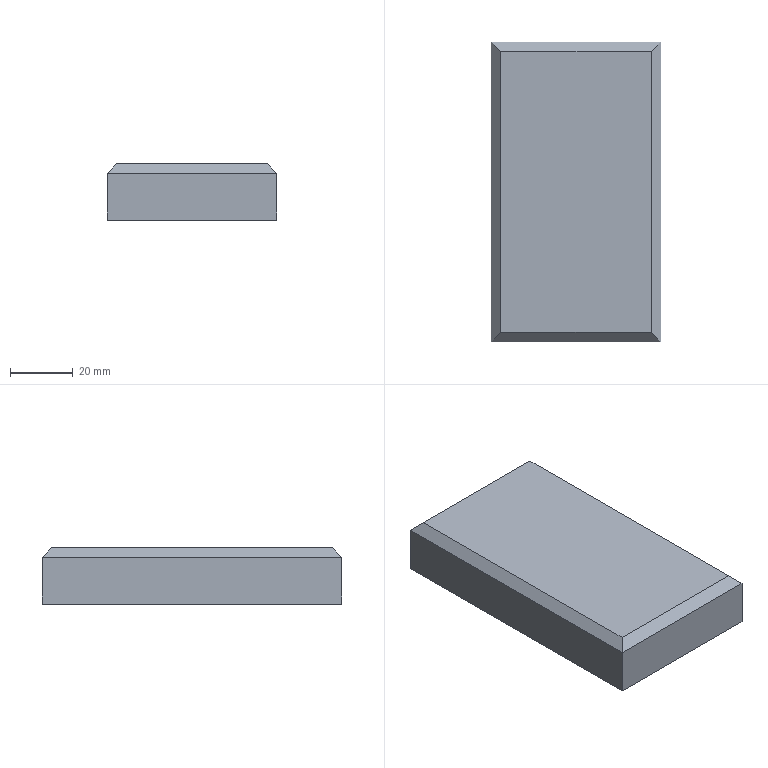Part | NX | 1 solid | 10 faces | box 54.267 x 95.886 x 18 mm | volume 92346 mm3 | plane 10
STEP:
#1=CARTESIAN_POINT('',(-11.284,-691.843,2485.086));
#2=VERTEX_POINT('',#1);
#3=CARTESIAN_POINT('',(-11.284,-691.843,2500.086));
#4=VERTEX_POINT('',#3);
#5=CARTESIAN_POINT('',(-11.284,-691.843,2485.086));
#6=DIRECTION('',(0.,0.,1.));
#7=VECTOR('',#6,1.);
#8=LINE('',#5,#7);
#9=EDGE_CURVE('',#2,#4,#8,.T.);
#10=ORIENTED_EDGE('',*,*,#9,.T.);
#11=CARTESIAN_POINT('',(-11.284,-595.957,2500.086));
#12=VERTEX_POINT('',#11);
#13=CARTESIAN_POINT('',(-11.284,-595.957,2500.086));
#14=DIRECTION('',(0.,1.,0.));
#15=VECTOR('',#14,1.);
#16=LINE('',#13,#15);
#17=EDGE_CURVE('',#4,#12,#16,.T.);
#18=ORIENTED_EDGE('',*,*,#17,.T.);
#19=CARTESIAN_POINT('',(-11.284,-595.957,2485.086));
#20=VERTEX_POINT('',#19);
#21=CARTESIAN_POINT('',(-11.284,-595.957,2485.086));
#22=DIRECTION('',(0.,0.,1.));
#23=VECTOR('',#22,1.);
#24=LINE('',#21,#23);
#25=EDGE_CURVE('',#20,#12,#24,.T.);
#26=ORIENTED_EDGE('',*,*,#25,.F.);
#27=CARTESIAN_POINT('',(-11.284,-595.957,2485.086));
#28=DIRECTION('',(0.,-1.,0.));
#29=VECTOR('',#28,1.);
#30=LINE('',#27,#29);
#31=EDGE_CURVE('',#20,#2,#30,.T.);
#32=ORIENTED_EDGE('',*,*,#31,.T.);
#33=EDGE_LOOP('',(#10,#18,#26,#32));
#34=FACE_OUTER_BOUND('',#33,.T.);
#35=CARTESIAN_POINT('',(-11.284,-595.957,2485.086));
#36=DIRECTION('',(-1.,0.,0.));
#37=DIRECTION('',(0.,-1.,0.));
#38=AXIS2_PLACEMENT_3D('',#35,#36,#37);
#39=PLANE('',#38);
#40=ADVANCED_FACE('',(#34),#39,.T.);
#41=ORIENTED_EDGE('',*,*,#25,.T.);
#42=CARTESIAN_POINT('',(42.983,-595.957,2500.086));
#43=VERTEX_POINT('',#42);
#44=CARTESIAN_POINT('',(-11.284,-595.957,2500.086));
#45=DIRECTION('',(1.,0.,0.));
#46=VECTOR('',#45,1.);
#47=LINE('',#44,#46);
#48=EDGE_CURVE('',#12,#43,#47,.T.);
#49=ORIENTED_EDGE('',*,*,#48,.T.);
#50=CARTESIAN_POINT('',(42.983,-595.957,2485.086));
#51=VERTEX_POINT('',#50);
#52=CARTESIAN_POINT('',(42.983,-595.957,2485.086));
#53=DIRECTION('',(0.,0.,1.));
#54=VECTOR('',#53,1.);
#55=LINE('',#52,#54);
#56=EDGE_CURVE('',#51,#43,#55,.T.);
#57=ORIENTED_EDGE('',*,*,#56,.F.);
#58=CARTESIAN_POINT('',(-11.284,-595.957,2485.086));
#59=DIRECTION('',(-1.,0.,0.));
#60=VECTOR('',#59,1.);
#61=LINE('',#58,#60);
#62=EDGE_CURVE('',#51,#20,#61,.T.);
#63=ORIENTED_EDGE('',*,*,#62,.T.);
#64=EDGE_LOOP('',(#41,#49,#57,#63));
#65=FACE_OUTER_BOUND('',#64,.T.);
#66=CARTESIAN_POINT('',(-11.284,-595.957,2485.086));
#67=DIRECTION('',(0.,1.,0.));
#68=DIRECTION('',(0.,0.,1.));
#69=AXIS2_PLACEMENT_3D('',#66,#67,#68);
#70=PLANE('',#69);
#71=ADVANCED_FACE('',(#65),#70,.T.);
#72=ORIENTED_EDGE('',*,*,#56,.T.);
#73=CARTESIAN_POINT('',(42.983,-691.843,2500.086));
#74=VERTEX_POINT('',#73);
#75=CARTESIAN_POINT('',(42.983,-595.957,2500.086));
#76=DIRECTION('',(0.,-1.,0.));
#77=VECTOR('',#76,1.);
#78=LINE('',#75,#77);
#79=EDGE_CURVE('',#43,#74,#78,.T.);
#80=ORIENTED_EDGE('',*,*,#79,.T.);
#81=CARTESIAN_POINT('',(42.983,-691.843,2485.086));
#82=VERTEX_POINT('',#81);
#83=CARTESIAN_POINT('',(42.983,-691.843,2485.086));
#84=DIRECTION('',(0.,0.,1.));
#85=VECTOR('',#84,1.);
#86=LINE('',#83,#85);
#87=EDGE_CURVE('',#82,#74,#86,.T.);
#88=ORIENTED_EDGE('',*,*,#87,.F.);
#89=CARTESIAN_POINT('',(42.983,-595.957,2485.086));
#90=DIRECTION('',(0.,1.,0.));
#91=VECTOR('',#90,1.);
#92=LINE('',#89,#91);
#93=EDGE_CURVE('',#82,#51,#92,.T.);
#94=ORIENTED_EDGE('',*,*,#93,.T.);
#95=EDGE_LOOP('',(#72,#80,#88,#94));
#96=FACE_OUTER_BOUND('',#95,.T.);
#97=CARTESIAN_POINT('',(42.983,-595.957,2485.086));
#98=DIRECTION('',(1.,0.,0.));
#99=DIRECTION('',(0.,0.,-1.));
#100=AXIS2_PLACEMENT_3D('',#97,#98,#99);
#101=PLANE('',#100);
#102=ADVANCED_FACE('',(#96),#101,.T.);
#103=ORIENTED_EDGE('',*,*,#87,.T.);
#104=CARTESIAN_POINT('',(-11.284,-691.843,2500.086));
#105=DIRECTION('',(-1.,0.,0.));
#106=VECTOR('',#105,1.);
#107=LINE('',#104,#106);
#108=EDGE_CURVE('',#74,#4,#107,.T.);
#109=ORIENTED_EDGE('',*,*,#108,.T.);
#110=ORIENTED_EDGE('',*,*,#9,.F.);
#111=CARTESIAN_POINT('',(-11.284,-691.843,2485.086));
#112=DIRECTION('',(1.,0.,0.));
#113=VECTOR('',#112,1.);
#114=LINE('',#111,#113);
#115=EDGE_CURVE('',#2,#82,#114,.T.);
#116=ORIENTED_EDGE('',*,*,#115,.T.);
#117=EDGE_LOOP('',(#103,#109,#110,#116));
#118=FACE_OUTER_BOUND('',#117,.T.);
#119=CARTESIAN_POINT('',(-11.284,-691.843,2485.086));
#120=DIRECTION('',(0.,-1.,0.));
#121=DIRECTION('',(0.,0.,-1.));
#122=AXIS2_PLACEMENT_3D('',#119,#120,#121);
#123=PLANE('',#122);
#124=ADVANCED_FACE('',(#118),#123,.T.);
#125=ORIENTED_EDGE('',*,*,#31,.F.);
#126=ORIENTED_EDGE('',*,*,#62,.F.);
#127=ORIENTED_EDGE('',*,*,#93,.F.);
#128=ORIENTED_EDGE('',*,*,#115,.F.);
#129=EDGE_LOOP('',(#125,#126,#127,#128));
#130=FACE_OUTER_BOUND('',#129,.T.);
#131=CARTESIAN_POINT('',(-11.284,-691.843,2485.086));
#132=DIRECTION('',(0.,0.,1.));
#133=DIRECTION('',(1.,0.,0.));
#134=AXIS2_PLACEMENT_3D('',#131,#132,#133);
#135=PLANE('',#134);
#136=ADVANCED_FACE('',(#130),#135,.F.);
#137=CARTESIAN_POINT('',(39.983,-688.843,2503.086));
#138=VERTEX_POINT('',#137);
#139=CARTESIAN_POINT('',(39.983,-598.957,2503.086));
#140=VERTEX_POINT('',#139);
#141=CARTESIAN_POINT('',(39.983,-691.843,2503.086));
#142=DIRECTION('',(0.,1.,0.));
#143=VECTOR('',#142,1.);
#144=LINE('',#141,#143);
#145=EDGE_CURVE('',#138,#140,#144,.T.);
#146=ORIENTED_EDGE('',*,*,#145,.T.);
#147=CARTESIAN_POINT('',(-8.284,-598.957,2503.086));
#148=VERTEX_POINT('',#147);
#149=CARTESIAN_POINT('',(-11.284,-598.957,2503.086));
#150=DIRECTION('',(-1.,0.,0.));
#151=VECTOR('',#150,1.);
#152=LINE('',#149,#151);
#153=EDGE_CURVE('',#140,#148,#152,.T.);
#154=ORIENTED_EDGE('',*,*,#153,.T.);
#155=CARTESIAN_POINT('',(-8.284,-688.843,2503.086));
#156=VERTEX_POINT('',#155);
#157=CARTESIAN_POINT('',(-8.284,-691.843,2503.086));
#158=DIRECTION('',(0.,-1.,0.));
#159=VECTOR('',#158,1.);
#160=LINE('',#157,#159);
#161=EDGE_CURVE('',#148,#156,#160,.T.);
#162=ORIENTED_EDGE('',*,*,#161,.T.);
#163=CARTESIAN_POINT('',(-11.284,-688.843,2503.086));
#164=DIRECTION('',(1.,0.,0.));
#165=VECTOR('',#164,1.);
#166=LINE('',#163,#165);
#167=EDGE_CURVE('',#156,#138,#166,.T.);
#168=ORIENTED_EDGE('',*,*,#167,.T.);
#169=EDGE_LOOP('',(#146,#154,#162,#168));
#170=FACE_OUTER_BOUND('',#169,.T.);
#171=CARTESIAN_POINT('',(-11.284,-691.843,2503.086));
#172=DIRECTION('',(0.,0.,1.));
#173=DIRECTION('',(1.,0.,0.));
#174=AXIS2_PLACEMENT_3D('',#171,#172,#173);
#175=PLANE('',#174);
#176=ADVANCED_FACE('',(#170),#175,.T.);
#177=CARTESIAN_POINT('',(-9.284,-689.843,2502.086));
#178=DIRECTION('',(0.5774,0.5774,0.5774));
#179=VECTOR('',#178,1.);
#180=LINE('',#177,#179);
#181=EDGE_CURVE('',#4,#156,#180,.T.);
#182=ORIENTED_EDGE('',*,*,#181,.F.);
#183=ORIENTED_EDGE('',*,*,#108,.F.);
#184=CARTESIAN_POINT('',(22.894,-671.754,2520.175));
#185=DIRECTION('',(0.5774,-0.5774,-0.5774));
#186=VECTOR('',#185,1.);
#187=LINE('',#184,#186);
#188=EDGE_CURVE('',#138,#74,#187,.T.);
#189=ORIENTED_EDGE('',*,*,#188,.F.);
#190=ORIENTED_EDGE('',*,*,#167,.F.);
#191=EDGE_LOOP('',(#182,#183,#189,#190));
#192=FACE_OUTER_BOUND('',#191,.T.);
#193=CARTESIAN_POINT('',(-11.284,-688.843,2503.086));
#194=DIRECTION('',(0.,0.7071,-0.7071));
#195=DIRECTION('',(0.,0.7071,0.7071));
#196=AXIS2_PLACEMENT_3D('',#193,#194,#195);
#197=PLANE('',#196);
#198=ADVANCED_FACE('',(#192),#197,.F.);
#199=ORIENTED_EDGE('',*,*,#188,.T.);
#200=ORIENTED_EDGE('',*,*,#79,.F.);
#201=CARTESIAN_POINT('',(9.021,-629.919,2534.048));
#202=DIRECTION('',(0.5774,0.5774,-0.5774));
#203=VECTOR('',#202,1.);
#204=LINE('',#201,#203);
#205=EDGE_CURVE('',#140,#43,#204,.T.);
#206=ORIENTED_EDGE('',*,*,#205,.F.);
#207=ORIENTED_EDGE('',*,*,#145,.F.);
#208=EDGE_LOOP('',(#199,#200,#206,#207));
#209=FACE_OUTER_BOUND('',#208,.T.);
#210=CARTESIAN_POINT('',(39.983,-691.843,2503.086));
#211=DIRECTION('',(-0.7071,0.,-0.7071));
#212=DIRECTION('',(-0.7071,0.,0.7071));
#213=AXIS2_PLACEMENT_3D('',#210,#211,#212);
#214=PLANE('',#213);
#215=ADVANCED_FACE('',(#209),#214,.F.);
#216=ORIENTED_EDGE('',*,*,#181,.T.);
#217=ORIENTED_EDGE('',*,*,#161,.F.);
#218=CARTESIAN_POINT('',(22.678,-629.919,2534.048));
#219=DIRECTION('',(0.5774,-0.5774,0.5774));
#220=VECTOR('',#219,1.);
#221=LINE('',#218,#220);
#222=EDGE_CURVE('',#12,#148,#221,.T.);
#223=ORIENTED_EDGE('',*,*,#222,.F.);
#224=ORIENTED_EDGE('',*,*,#17,.F.);
#225=EDGE_LOOP('',(#216,#217,#223,#224));
#226=FACE_OUTER_BOUND('',#225,.T.);
#227=CARTESIAN_POINT('',(-8.284,-691.843,2503.086));
#228=DIRECTION('',(0.7071,0.,-0.7071));
#229=DIRECTION('',(-0.7071,0.,-0.7071));
#230=AXIS2_PLACEMENT_3D('',#227,#228,#229);
#231=PLANE('',#230);
#232=ADVANCED_FACE('',(#226),#231,.F.);
#233=ORIENTED_EDGE('',*,*,#205,.T.);
#234=ORIENTED_EDGE('',*,*,#48,.F.);
#235=ORIENTED_EDGE('',*,*,#222,.T.);
#236=ORIENTED_EDGE('',*,*,#153,.F.);
#237=EDGE_LOOP('',(#233,#234,#235,#236));
#238=FACE_OUTER_BOUND('',#237,.T.);
#239=CARTESIAN_POINT('',(-11.284,-598.957,2503.086));
#240=DIRECTION('',(0.,-0.7071,-0.7071));
#241=DIRECTION('',(0.,0.7071,-0.7071));
#242=AXIS2_PLACEMENT_3D('',#239,#240,#241);
#243=PLANE('',#242);
#244=ADVANCED_FACE('',(#238),#243,.F.);
#245=CLOSED_SHELL('',(#40,#71,#102,#124,#136,#176,#198,#215,#232,#244));
#246=MANIFOLD_SOLID_BREP('',#245);
#247=(LENGTH_UNIT()NAMED_UNIT(*)SI_UNIT(.MILLI.,.METRE.));
#248=UNCERTAINTY_MEASURE_WITH_UNIT(LENGTH_MEASURE(0.00002),#247,'','');
#249=(NAMED_UNIT(*)PLANE_ANGLE_UNIT()SI_UNIT($,.RADIAN.));
#250=PLANE_ANGLE_MEASURE_WITH_UNIT(PLANE_ANGLE_MEASURE(0.01745),#249);
#251=DIMENSIONAL_EXPONENTS(0.,0.,0.,0.,0.,0.,0.);
#252=(CONVERSION_BASED_UNIT('DEGREE',#250)NAMED_UNIT(#251)PLANE_ANGLE_UNIT());
#253=(NAMED_UNIT(*)SI_UNIT($,.STERADIAN.)SOLID_ANGLE_UNIT());
#254=(GEOMETRIC_REPRESENTATION_CONTEXT(3)GLOBAL_UNCERTAINTY_ASSIGNED_CONTEXT((#248))GLOBAL_UNIT_ASSIGNED_CONTEXT((#247,#252,#253))REPRESENTATION_CONTEXT('',''));
#255=ADVANCED_BREP_SHAPE_REPRESENTATION('',(#246),#254);